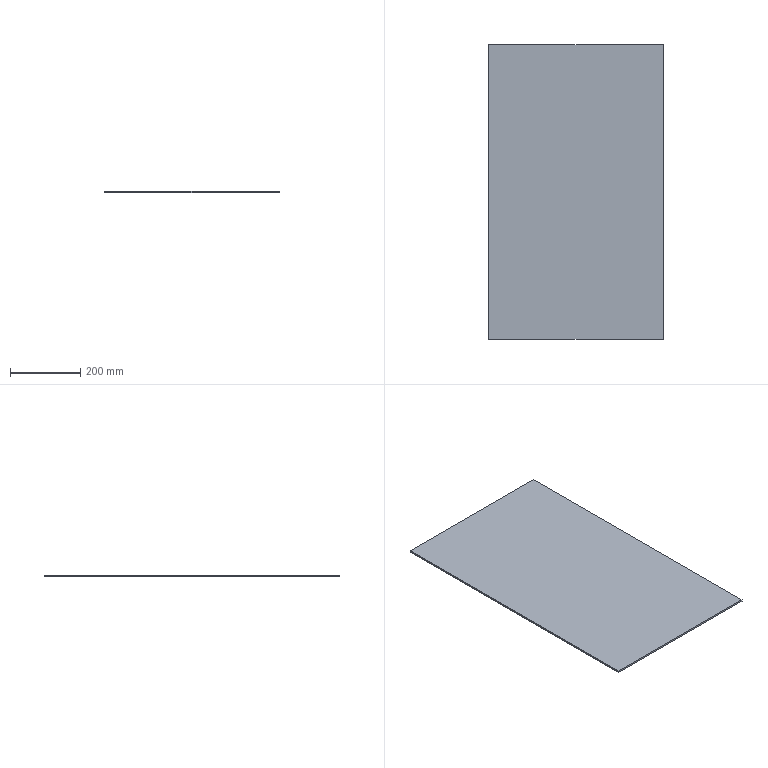Part | SolidWorks | features Extrusion 1, HoleWzd 1 | 1 solid | 6 faces | box 499 x 842 x 5 mm | volume 2100790 mm3 | plane 6
STEP:
#1=CARTESIAN_POINT('',(249.5,-421.,0.));
#2=VERTEX_POINT('',#1);
#3=CARTESIAN_POINT('',(249.5,421.,0.));
#4=VERTEX_POINT('',#3);
#5=CARTESIAN_POINT('',(249.5,421.,0.));
#6=DIRECTION('',(0.,1.,0.));
#7=VECTOR('',#6,1000.);
#8=LINE('',#5,#7);
#9=EDGE_CURVE('',#2,#4,#8,.T.);
#10=ORIENTED_EDGE('',*,*,#9,.T.);
#11=CARTESIAN_POINT('',(249.5,421.,5.));
#12=VERTEX_POINT('',#11);
#13=CARTESIAN_POINT('',(249.5,421.,5.));
#14=DIRECTION('',(0.,0.,-1.));
#15=VECTOR('',#14,1000.);
#16=LINE('',#13,#15);
#17=EDGE_CURVE('',#12,#4,#16,.T.);
#18=ORIENTED_EDGE('',*,*,#17,.F.);
#19=CARTESIAN_POINT('',(249.5,-421.,5.));
#20=VERTEX_POINT('',#19);
#21=CARTESIAN_POINT('',(249.5,421.,5.));
#22=DIRECTION('',(0.,1.,0.));
#23=VECTOR('',#22,1000.);
#24=LINE('',#21,#23);
#25=EDGE_CURVE('',#20,#12,#24,.T.);
#26=ORIENTED_EDGE('',*,*,#25,.F.);
#27=CARTESIAN_POINT('',(249.5,-421.,5.));
#28=DIRECTION('',(0.,0.,-1.));
#29=VECTOR('',#28,1000.);
#30=LINE('',#27,#29);
#31=EDGE_CURVE('',#20,#2,#30,.T.);
#32=ORIENTED_EDGE('',*,*,#31,.T.);
#33=EDGE_LOOP('',(#10,#18,#26,#32));
#34=FACE_OUTER_BOUND('',#33,.T.);
#35=CARTESIAN_POINT('',(249.5,421.,5.));
#36=DIRECTION('',(-1.,0.,0.));
#37=DIRECTION('',(0.,-1.,0.));
#38=AXIS2_PLACEMENT_3D('',#35,#36,#37);
#39=PLANE('',#38);
#40=ADVANCED_FACE('',(#34),#39,.F.);
#41=CARTESIAN_POINT('',(-249.5,421.,0.));
#42=VERTEX_POINT('',#41);
#43=CARTESIAN_POINT('',(-249.5,421.,0.));
#44=DIRECTION('',(-1.,0.,0.));
#45=VECTOR('',#44,1000.);
#46=LINE('',#43,#45);
#47=EDGE_CURVE('',#4,#42,#46,.T.);
#48=ORIENTED_EDGE('',*,*,#47,.T.);
#49=CARTESIAN_POINT('',(-249.5,421.,5.));
#50=VERTEX_POINT('',#49);
#51=CARTESIAN_POINT('',(-249.5,421.,5.));
#52=DIRECTION('',(0.,0.,-1.));
#53=VECTOR('',#52,1000.);
#54=LINE('',#51,#53);
#55=EDGE_CURVE('',#50,#42,#54,.T.);
#56=ORIENTED_EDGE('',*,*,#55,.F.);
#57=CARTESIAN_POINT('',(-249.5,421.,5.));
#58=DIRECTION('',(-1.,0.,0.));
#59=VECTOR('',#58,1000.);
#60=LINE('',#57,#59);
#61=EDGE_CURVE('',#12,#50,#60,.T.);
#62=ORIENTED_EDGE('',*,*,#61,.F.);
#63=ORIENTED_EDGE('',*,*,#17,.T.);
#64=EDGE_LOOP('',(#48,#56,#62,#63));
#65=FACE_OUTER_BOUND('',#64,.T.);
#66=CARTESIAN_POINT('',(-249.5,421.,5.));
#67=DIRECTION('',(0.,-1.,0.));
#68=DIRECTION('',(0.,0.,-1.));
#69=AXIS2_PLACEMENT_3D('',#66,#67,#68);
#70=PLANE('',#69);
#71=ADVANCED_FACE('',(#65),#70,.F.);
#72=CARTESIAN_POINT('',(-249.5,-421.,0.));
#73=VERTEX_POINT('',#72);
#74=CARTESIAN_POINT('',(-249.5,421.,0.));
#75=DIRECTION('',(0.,-1.,0.));
#76=VECTOR('',#75,1000.);
#77=LINE('',#74,#76);
#78=EDGE_CURVE('',#42,#73,#77,.T.);
#79=ORIENTED_EDGE('',*,*,#78,.T.);
#80=CARTESIAN_POINT('',(-249.5,-421.,5.));
#81=VERTEX_POINT('',#80);
#82=CARTESIAN_POINT('',(-249.5,-421.,5.));
#83=DIRECTION('',(0.,0.,-1.));
#84=VECTOR('',#83,1000.);
#85=LINE('',#82,#84);
#86=EDGE_CURVE('',#81,#73,#85,.T.);
#87=ORIENTED_EDGE('',*,*,#86,.F.);
#88=CARTESIAN_POINT('',(-249.5,421.,5.));
#89=DIRECTION('',(0.,-1.,0.));
#90=VECTOR('',#89,1000.);
#91=LINE('',#88,#90);
#92=EDGE_CURVE('',#50,#81,#91,.T.);
#93=ORIENTED_EDGE('',*,*,#92,.F.);
#94=ORIENTED_EDGE('',*,*,#55,.T.);
#95=EDGE_LOOP('',(#79,#87,#93,#94));
#96=FACE_OUTER_BOUND('',#95,.T.);
#97=CARTESIAN_POINT('',(-249.5,421.,5.));
#98=DIRECTION('',(1.,0.,0.));
#99=DIRECTION('',(0.,1.,0.));
#100=AXIS2_PLACEMENT_3D('',#97,#98,#99);
#101=PLANE('',#100);
#102=ADVANCED_FACE('',(#96),#101,.F.);
#103=CARTESIAN_POINT('',(-249.5,-421.,0.));
#104=DIRECTION('',(1.,0.,0.));
#105=VECTOR('',#104,1000.);
#106=LINE('',#103,#105);
#107=EDGE_CURVE('',#73,#2,#106,.T.);
#108=ORIENTED_EDGE('',*,*,#107,.T.);
#109=ORIENTED_EDGE('',*,*,#31,.F.);
#110=CARTESIAN_POINT('',(-249.5,-421.,5.));
#111=DIRECTION('',(1.,0.,0.));
#112=VECTOR('',#111,1000.);
#113=LINE('',#110,#112);
#114=EDGE_CURVE('',#81,#20,#113,.T.);
#115=ORIENTED_EDGE('',*,*,#114,.F.);
#116=ORIENTED_EDGE('',*,*,#86,.T.);
#117=EDGE_LOOP('',(#108,#109,#115,#116));
#118=FACE_OUTER_BOUND('',#117,.T.);
#119=CARTESIAN_POINT('',(-249.5,-421.,5.));
#120=DIRECTION('',(0.,1.,0.));
#121=DIRECTION('',(0.,0.,1.));
#122=AXIS2_PLACEMENT_3D('',#119,#120,#121);
#123=PLANE('',#122);
#124=ADVANCED_FACE('',(#118),#123,.F.);
#125=ORIENTED_EDGE('',*,*,#25,.T.);
#126=ORIENTED_EDGE('',*,*,#61,.T.);
#127=ORIENTED_EDGE('',*,*,#92,.T.);
#128=ORIENTED_EDGE('',*,*,#114,.T.);
#129=EDGE_LOOP('',(#125,#126,#127,#128));
#130=FACE_OUTER_BOUND('',#129,.T.);
#131=CARTESIAN_POINT('',(0.,0.,5.));
#132=DIRECTION('',(0.,0.,1.));
#133=DIRECTION('',(1.,0.,0.));
#134=AXIS2_PLACEMENT_3D('',#131,#132,#133);
#135=PLANE('',#134);
#136=ADVANCED_FACE('',(#130),#135,.T.);
#137=ORIENTED_EDGE('',*,*,#9,.F.);
#138=ORIENTED_EDGE('',*,*,#107,.F.);
#139=ORIENTED_EDGE('',*,*,#78,.F.);
#140=ORIENTED_EDGE('',*,*,#47,.F.);
#141=EDGE_LOOP('',(#137,#138,#139,#140));
#142=FACE_OUTER_BOUND('',#141,.T.);
#143=CARTESIAN_POINT('',(0.,0.,0.));
#144=DIRECTION('',(0.,0.,1.));
#145=DIRECTION('',(1.,0.,0.));
#146=AXIS2_PLACEMENT_3D('',#143,#144,#145);
#147=PLANE('',#146);
#148=ADVANCED_FACE('',(#142),#147,.F.);
#149=CLOSED_SHELL('',(#40,#71,#102,#124,#136,#148));
#150=MANIFOLD_SOLID_BREP('',#149);
#151=CARTESIAN_POINT('',(0.,0.,0.));
#152=DIRECTION('',(0.,0.,1.));
#153=DIRECTION('',(1.,0.,0.));
#154=AXIS2_PLACEMENT_3D('',#151,#152,#153);
#155=(LENGTH_UNIT()NAMED_UNIT(*)SI_UNIT(.MILLI.,.METRE.));
#156=UNCERTAINTY_MEASURE_WITH_UNIT(LENGTH_MEASURE(0.00001),#155,'','');
#157=(NAMED_UNIT(*)PLANE_ANGLE_UNIT()SI_UNIT($,.RADIAN.));
#158=(NAMED_UNIT(*)SI_UNIT($,.STERADIAN.)SOLID_ANGLE_UNIT());
#159=(GEOMETRIC_REPRESENTATION_CONTEXT(3)GLOBAL_UNCERTAINTY_ASSIGNED_CONTEXT((#156))GLOBAL_UNIT_ASSIGNED_CONTEXT((#155,#157,#158))REPRESENTATION_CONTEXT('',''));
#160=ADVANCED_BREP_SHAPE_REPRESENTATION('',(#150,#154),#159);